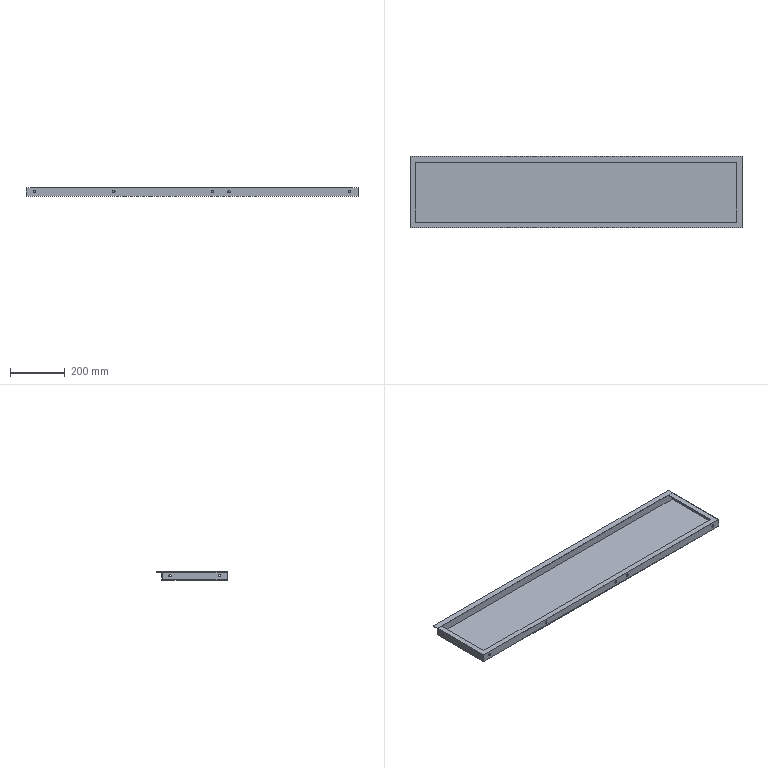Part | SolidWorks | features ICE 3, Extrusion 1, Shell 1 | 1 solid | 35 faces | box 1210 x 260 x 30 mm | volume 849119 mm3 | cylinder 18 | plane 17 | commonest cylinder face diameters 9 x18
STEP:
#1=CARTESIAN_POINT('',(740.,0.,11.5));
#2=VERTEX_POINT('',#1);
#3=CARTESIAN_POINT('',(740.,0.,20.5));
#4=VERTEX_POINT('',#3);
#5=CARTESIAN_POINT('',(740.,0.,16.));
#6=DIRECTION('',(0.,1.,0.));
#7=DIRECTION('',(0.,0.,1.));
#8=AXIS2_PLACEMENT_3D('',#5,#6,#7);
#9=CIRCLE('',#8,4.5);
#10=EDGE_CURVE('',#2,#4,#9,.T.);
#11=ORIENTED_EDGE('',*,*,#10,.F.);
#12=CARTESIAN_POINT('',(740.,2.,11.5));
#13=VERTEX_POINT('',#12);
#14=CARTESIAN_POINT('',(740.,-43.,11.5));
#15=DIRECTION('',(0.,1.,0.));
#16=VECTOR('',#15,1000.);
#17=LINE('',#14,#16);
#18=EDGE_CURVE('',#2,#13,#17,.T.);
#19=ORIENTED_EDGE('',*,*,#18,.T.);
#20=CARTESIAN_POINT('',(740.,2.,20.5));
#21=VERTEX_POINT('',#20);
#22=CARTESIAN_POINT('',(740.,2.,16.));
#23=DIRECTION('',(0.,1.,0.));
#24=DIRECTION('',(0.,0.,1.));
#25=AXIS2_PLACEMENT_3D('',#22,#23,#24);
#26=CIRCLE('',#25,4.5);
#27=EDGE_CURVE('',#13,#21,#26,.T.);
#28=ORIENTED_EDGE('',*,*,#27,.T.);
#29=CARTESIAN_POINT('',(740.,-43.,20.5));
#30=DIRECTION('',(0.,1.,0.));
#31=VECTOR('',#30,1000.);
#32=LINE('',#29,#31);
#33=EDGE_CURVE('',#4,#21,#32,.T.);
#34=ORIENTED_EDGE('',*,*,#33,.F.);
#35=EDGE_LOOP('',(#11,#19,#28,#34));
#36=FACE_OUTER_BOUND('',#35,.T.);
#37=CARTESIAN_POINT('',(740.,-43.,16.));
#38=DIRECTION('',(0.,1.,0.));
#39=DIRECTION('',(0.,0.,1.));
#40=AXIS2_PLACEMENT_3D('',#37,#38,#39);
#41=CYLINDRICAL_SURFACE('',#40,4.5);
#42=ADVANCED_FACE('',(#36),#41,.F.);
#43=CARTESIAN_POINT('',(320.,0.,11.5));
#44=VERTEX_POINT('',#43);
#45=CARTESIAN_POINT('',(320.,0.,20.5));
#46=VERTEX_POINT('',#45);
#47=CARTESIAN_POINT('',(320.,0.,16.));
#48=DIRECTION('',(0.,1.,0.));
#49=DIRECTION('',(0.,0.,1.));
#50=AXIS2_PLACEMENT_3D('',#47,#48,#49);
#51=CIRCLE('',#50,4.5);
#52=EDGE_CURVE('',#44,#46,#51,.T.);
#53=ORIENTED_EDGE('',*,*,#52,.F.);
#54=CARTESIAN_POINT('',(320.,2.,11.5));
#55=VERTEX_POINT('',#54);
#56=CARTESIAN_POINT('',(320.,-43.,11.5));
#57=DIRECTION('',(0.,1.,0.));
#58=VECTOR('',#57,1000.);
#59=LINE('',#56,#58);
#60=EDGE_CURVE('',#44,#55,#59,.T.);
#61=ORIENTED_EDGE('',*,*,#60,.T.);
#62=CARTESIAN_POINT('',(320.,2.,20.5));
#63=VERTEX_POINT('',#62);
#64=CARTESIAN_POINT('',(320.,2.,16.));
#65=DIRECTION('',(0.,1.,0.));
#66=DIRECTION('',(0.,0.,1.));
#67=AXIS2_PLACEMENT_3D('',#64,#65,#66);
#68=CIRCLE('',#67,4.5);
#69=EDGE_CURVE('',#55,#63,#68,.T.);
#70=ORIENTED_EDGE('',*,*,#69,.T.);
#71=CARTESIAN_POINT('',(320.,-43.,20.5));
#72=DIRECTION('',(0.,1.,0.));
#73=VECTOR('',#72,1000.);
#74=LINE('',#71,#73);
#75=EDGE_CURVE('',#46,#63,#74,.T.);
#76=ORIENTED_EDGE('',*,*,#75,.F.);
#77=EDGE_LOOP('',(#53,#61,#70,#76));
#78=FACE_OUTER_BOUND('',#77,.T.);
#79=CARTESIAN_POINT('',(320.,-43.,16.));
#80=DIRECTION('',(0.,1.,0.));
#81=DIRECTION('',(0.,0.,1.));
#82=AXIS2_PLACEMENT_3D('',#79,#80,#81);
#83=CYLINDRICAL_SURFACE('',#82,4.5);
#84=ADVANCED_FACE('',(#78),#83,.F.);
#85=CARTESIAN_POINT('',(680.,0.,11.5));
#86=VERTEX_POINT('',#85);
#87=CARTESIAN_POINT('',(680.,0.,20.5));
#88=VERTEX_POINT('',#87);
#89=CARTESIAN_POINT('',(680.,0.,16.));
#90=DIRECTION('',(0.,1.,0.));
#91=DIRECTION('',(0.,0.,1.));
#92=AXIS2_PLACEMENT_3D('',#89,#90,#91);
#93=CIRCLE('',#92,4.5);
#94=EDGE_CURVE('',#86,#88,#93,.T.);
#95=ORIENTED_EDGE('',*,*,#94,.F.);
#96=CARTESIAN_POINT('',(680.,2.,11.5));
#97=VERTEX_POINT('',#96);
#98=CARTESIAN_POINT('',(680.,-43.,11.5));
#99=DIRECTION('',(0.,1.,0.));
#100=VECTOR('',#99,1000.);
#101=LINE('',#98,#100);
#102=EDGE_CURVE('',#86,#97,#101,.T.);
#103=ORIENTED_EDGE('',*,*,#102,.T.);
#104=CARTESIAN_POINT('',(680.,2.,20.5));
#105=VERTEX_POINT('',#104);
#106=CARTESIAN_POINT('',(680.,2.,16.));
#107=DIRECTION('',(0.,1.,0.));
#108=DIRECTION('',(0.,0.,1.));
#109=AXIS2_PLACEMENT_3D('',#106,#107,#108);
#110=CIRCLE('',#109,4.5);
#111=EDGE_CURVE('',#97,#105,#110,.T.);
#112=ORIENTED_EDGE('',*,*,#111,.T.);
#113=CARTESIAN_POINT('',(680.,-43.,20.5));
#114=DIRECTION('',(0.,1.,0.));
#115=VECTOR('',#114,1000.);
#116=LINE('',#113,#115);
#117=EDGE_CURVE('',#88,#105,#116,.T.);
#118=ORIENTED_EDGE('',*,*,#117,.F.);
#119=EDGE_LOOP('',(#95,#103,#112,#118));
#120=FACE_OUTER_BOUND('',#119,.T.);
#121=CARTESIAN_POINT('',(680.,-43.,16.));
#122=DIRECTION('',(0.,1.,0.));
#123=DIRECTION('',(0.,0.,1.));
#124=AXIS2_PLACEMENT_3D('',#121,#122,#123);
#125=CYLINDRICAL_SURFACE('',#124,4.5);
#126=ADVANCED_FACE('',(#120),#125,.F.);
#127=CARTESIAN_POINT('',(1180.,0.,11.5));
#128=VERTEX_POINT('',#127);
#129=CARTESIAN_POINT('',(1180.,0.,20.5));
#130=VERTEX_POINT('',#129);
#131=CARTESIAN_POINT('',(1180.,0.,16.));
#132=DIRECTION('',(0.,1.,0.));
#133=DIRECTION('',(0.,0.,1.));
#134=AXIS2_PLACEMENT_3D('',#131,#132,#133);
#135=CIRCLE('',#134,4.5);
#136=EDGE_CURVE('',#128,#130,#135,.T.);
#137=ORIENTED_EDGE('',*,*,#136,.F.);
#138=CARTESIAN_POINT('',(1180.,2.,11.5));
#139=VERTEX_POINT('',#138);
#140=CARTESIAN_POINT('',(1180.,-43.,11.5));
#141=DIRECTION('',(0.,1.,0.));
#142=VECTOR('',#141,1000.);
#143=LINE('',#140,#142);
#144=EDGE_CURVE('',#128,#139,#143,.T.);
#145=ORIENTED_EDGE('',*,*,#144,.T.);
#146=CARTESIAN_POINT('',(1180.,2.,20.5));
#147=VERTEX_POINT('',#146);
#148=CARTESIAN_POINT('',(1180.,2.,16.));
#149=DIRECTION('',(0.,1.,0.));
#150=DIRECTION('',(0.,0.,1.));
#151=AXIS2_PLACEMENT_3D('',#148,#149,#150);
#152=CIRCLE('',#151,4.5);
#153=EDGE_CURVE('',#139,#147,#152,.T.);
#154=ORIENTED_EDGE('',*,*,#153,.T.);
#155=CARTESIAN_POINT('',(1180.,-43.,20.5));
#156=DIRECTION('',(0.,1.,0.));
#157=VECTOR('',#156,1000.);
#158=LINE('',#155,#157);
#159=EDGE_CURVE('',#130,#147,#158,.T.);
#160=ORIENTED_EDGE('',*,*,#159,.F.);
#161=EDGE_LOOP('',(#137,#145,#154,#160));
#162=FACE_OUTER_BOUND('',#161,.T.);
#163=CARTESIAN_POINT('',(1180.,-43.,16.));
#164=DIRECTION('',(0.,1.,0.));
#165=DIRECTION('',(0.,0.,1.));
#166=AXIS2_PLACEMENT_3D('',#163,#164,#165);
#167=CYLINDRICAL_SURFACE('',#166,4.5);
#168=ADVANCED_FACE('',(#162),#167,.F.);
#169=CARTESIAN_POINT('',(30.,0.,11.5));
#170=VERTEX_POINT('',#169);
#171=CARTESIAN_POINT('',(30.,0.,20.5));
#172=VERTEX_POINT('',#171);
#173=CARTESIAN_POINT('',(30.,0.,16.));
#174=DIRECTION('',(0.,1.,0.));
#175=DIRECTION('',(0.,0.,1.));
#176=AXIS2_PLACEMENT_3D('',#173,#174,#175);
#177=CIRCLE('',#176,4.5);
#178=EDGE_CURVE('',#170,#172,#177,.T.);
#179=ORIENTED_EDGE('',*,*,#178,.F.);
#180=CARTESIAN_POINT('',(30.,2.,11.5));
#181=VERTEX_POINT('',#180);
#182=CARTESIAN_POINT('',(30.,-43.,11.5));
#183=DIRECTION('',(0.,1.,0.));
#184=VECTOR('',#183,1000.);
#185=LINE('',#182,#184);
#186=EDGE_CURVE('',#170,#181,#185,.T.);
#187=ORIENTED_EDGE('',*,*,#186,.T.);
#188=CARTESIAN_POINT('',(30.,2.,20.5));
#189=VERTEX_POINT('',#188);
#190=CARTESIAN_POINT('',(30.,2.,16.));
#191=DIRECTION('',(0.,1.,0.));
#192=DIRECTION('',(0.,0.,1.));
#193=AXIS2_PLACEMENT_3D('',#190,#191,#192);
#194=CIRCLE('',#193,4.5);
#195=EDGE_CURVE('',#181,#189,#194,.T.);
#196=ORIENTED_EDGE('',*,*,#195,.T.);
#197=CARTESIAN_POINT('',(30.,-43.,20.5));
#198=DIRECTION('',(0.,1.,0.));
#199=VECTOR('',#198,1000.);
#200=LINE('',#197,#199);
#201=EDGE_CURVE('',#172,#189,#200,.T.);
#202=ORIENTED_EDGE('',*,*,#201,.F.);
#203=EDGE_LOOP('',(#179,#187,#196,#202));
#204=FACE_OUTER_BOUND('',#203,.T.);
#205=CARTESIAN_POINT('',(30.,-43.,16.));
#206=DIRECTION('',(0.,1.,0.));
#207=DIRECTION('',(0.,0.,1.));
#208=AXIS2_PLACEMENT_3D('',#205,#206,#207);
#209=CYLINDRICAL_SURFACE('',#208,4.5);
#210=ADVANCED_FACE('',(#204),#209,.F.);
#211=CARTESIAN_POINT('',(0.,210.,20.5));
#212=VERTEX_POINT('',#211);
#213=CARTESIAN_POINT('',(0.,210.,11.5));
#214=VERTEX_POINT('',#213);
#215=CARTESIAN_POINT('',(0.,210.,16.));
#216=DIRECTION('',(1.,0.,0.));
#217=DIRECTION('',(0.,0.,-1.));
#218=AXIS2_PLACEMENT_3D('',#215,#216,#217);
#219=CIRCLE('',#218,4.5);
#220=EDGE_CURVE('',#212,#214,#219,.T.);
#221=ORIENTED_EDGE('',*,*,#220,.F.);
#222=CARTESIAN_POINT('',(2.,210.,20.5));
#223=VERTEX_POINT('',#222);
#224=CARTESIAN_POINT('',(-196.,210.,20.5));
#225=DIRECTION('',(1.,0.,0.));
#226=VECTOR('',#225,1000.);
#227=LINE('',#224,#226);
#228=EDGE_CURVE('',#212,#223,#227,.T.);
#229=ORIENTED_EDGE('',*,*,#228,.T.);
#230=CARTESIAN_POINT('',(2.,210.,11.5));
#231=VERTEX_POINT('',#230);
#232=CARTESIAN_POINT('',(2.,210.,16.));
#233=DIRECTION('',(1.,0.,0.));
#234=DIRECTION('',(0.,0.,-1.));
#235=AXIS2_PLACEMENT_3D('',#232,#233,#234);
#236=CIRCLE('',#235,4.5);
#237=EDGE_CURVE('',#223,#231,#236,.T.);
#238=ORIENTED_EDGE('',*,*,#237,.T.);
#239=CARTESIAN_POINT('',(-196.,210.,11.5));
#240=DIRECTION('',(1.,0.,0.));
#241=VECTOR('',#240,1000.);
#242=LINE('',#239,#241);
#243=EDGE_CURVE('',#214,#231,#242,.T.);
#244=ORIENTED_EDGE('',*,*,#243,.F.);
#245=EDGE_LOOP('',(#221,#229,#238,#244));
#246=FACE_OUTER_BOUND('',#245,.T.);
#247=CARTESIAN_POINT('',(-196.,210.,16.));
#248=DIRECTION('',(1.,0.,0.));
#249=DIRECTION('',(0.,0.,-1.));
#250=AXIS2_PLACEMENT_3D('',#247,#248,#249);
#251=CYLINDRICAL_SURFACE('',#250,4.5);
#252=ADVANCED_FACE('',(#246),#251,.F.);
#253=CARTESIAN_POINT('',(1208.,210.,11.5));
#254=VERTEX_POINT('',#253);
#255=CARTESIAN_POINT('',(1208.,210.,20.5));
#256=VERTEX_POINT('',#255);
#257=CARTESIAN_POINT('',(1208.,210.,16.));
#258=DIRECTION('',(-1.,0.,0.));
#259=DIRECTION('',(0.,0.,1.));
#260=AXIS2_PLACEMENT_3D('',#257,#258,#259);
#261=CIRCLE('',#260,4.5);
#262=EDGE_CURVE('',#254,#256,#261,.T.);
#263=ORIENTED_EDGE('',*,*,#262,.T.);
#264=CARTESIAN_POINT('',(1210.,210.,20.5));
#265=VERTEX_POINT('',#264);
#266=CARTESIAN_POINT('',(-196.,210.,20.5));
#267=DIRECTION('',(1.,0.,0.));
#268=VECTOR('',#267,1000.);
#269=LINE('',#266,#268);
#270=EDGE_CURVE('',#256,#265,#269,.T.);
#271=ORIENTED_EDGE('',*,*,#270,.T.);
#272=CARTESIAN_POINT('',(1210.,210.,11.5));
#273=VERTEX_POINT('',#272);
#274=CARTESIAN_POINT('',(1210.,210.,16.));
#275=DIRECTION('',(-1.,0.,0.));
#276=DIRECTION('',(0.,0.,1.));
#277=AXIS2_PLACEMENT_3D('',#274,#275,#276);
#278=CIRCLE('',#277,4.5);
#279=EDGE_CURVE('',#273,#265,#278,.T.);
#280=ORIENTED_EDGE('',*,*,#279,.F.);
#281=CARTESIAN_POINT('',(-196.,210.,11.5));
#282=DIRECTION('',(1.,0.,0.));
#283=VECTOR('',#282,1000.);
#284=LINE('',#281,#283);
#285=EDGE_CURVE('',#254,#273,#284,.T.);
#286=ORIENTED_EDGE('',*,*,#285,.F.);
#287=EDGE_LOOP('',(#263,#271,#280,#286));
#288=FACE_OUTER_BOUND('',#287,.T.);
#289=CARTESIAN_POINT('',(-196.,210.,16.));
#290=DIRECTION('',(1.,0.,0.));
#291=DIRECTION('',(0.,0.,-1.));
#292=AXIS2_PLACEMENT_3D('',#289,#290,#291);
#293=CYLINDRICAL_SURFACE('',#292,4.5);
#294=ADVANCED_FACE('',(#288),#293,.F.);
#295=CARTESIAN_POINT('',(0.,30.,20.5));
#296=VERTEX_POINT('',#295);
#297=CARTESIAN_POINT('',(0.,30.,11.5));
#298=VERTEX_POINT('',#297);
#299=CARTESIAN_POINT('',(0.,30.,16.));
#300=DIRECTION('',(1.,0.,0.));
#301=DIRECTION('',(0.,0.,-1.));
#302=AXIS2_PLACEMENT_3D('',#299,#300,#301);
#303=CIRCLE('',#302,4.5);
#304=EDGE_CURVE('',#296,#298,#303,.T.);
#305=ORIENTED_EDGE('',*,*,#304,.F.);
#306=CARTESIAN_POINT('',(2.,30.,20.5));
#307=VERTEX_POINT('',#306);
#308=CARTESIAN_POINT('',(-196.,30.,20.5));
#309=DIRECTION('',(1.,0.,0.));
#310=VECTOR('',#309,1000.);
#311=LINE('',#308,#310);
#312=EDGE_CURVE('',#296,#307,#311,.T.);
#313=ORIENTED_EDGE('',*,*,#312,.T.);
#314=CARTESIAN_POINT('',(2.,30.,11.5));
#315=VERTEX_POINT('',#314);
#316=CARTESIAN_POINT('',(2.,30.,16.));
#317=DIRECTION('',(1.,0.,0.));
#318=DIRECTION('',(0.,0.,-1.));
#319=AXIS2_PLACEMENT_3D('',#316,#317,#318);
#320=CIRCLE('',#319,4.5);
#321=EDGE_CURVE('',#307,#315,#320,.T.);
#322=ORIENTED_EDGE('',*,*,#321,.T.);
#323=CARTESIAN_POINT('',(-196.,30.,11.5));
#324=DIRECTION('',(1.,0.,0.));
#325=VECTOR('',#324,1000.);
#326=LINE('',#323,#325);
#327=EDGE_CURVE('',#298,#315,#326,.T.);
#328=ORIENTED_EDGE('',*,*,#327,.F.);
#329=EDGE_LOOP('',(#305,#313,#322,#328));
#330=FACE_OUTER_BOUND('',#329,.T.);
#331=CARTESIAN_POINT('',(-196.,30.,16.));
#332=DIRECTION('',(1.,0.,0.));
#333=DIRECTION('',(0.,0.,-1.));
#334=AXIS2_PLACEMENT_3D('',#331,#332,#333);
#335=CYLINDRICAL_SURFACE('',#334,4.5);
#336=ADVANCED_FACE('',(#330),#335,.F.);
#337=CARTESIAN_POINT('',(1208.,30.,11.5));
#338=VERTEX_POINT('',#337);
#339=CARTESIAN_POINT('',(1208.,30.,20.5));
#340=VERTEX_POINT('',#339);
#341=CARTESIAN_POINT('',(1208.,30.,16.));
#342=DIRECTION('',(-1.,0.,0.));
#343=DIRECTION('',(0.,0.,1.));
#344=AXIS2_PLACEMENT_3D('',#341,#342,#343);
#345=CIRCLE('',#344,4.5);
#346=EDGE_CURVE('',#338,#340,#345,.T.);
#347=ORIENTED_EDGE('',*,*,#346,.T.);
#348=CARTESIAN_POINT('',(1210.,30.,20.5));
#349=VERTEX_POINT('',#348);
#350=CARTESIAN_POINT('',(-196.,30.,20.5));
#351=DIRECTION('',(1.,0.,0.));
#352=VECTOR('',#351,1000.);
#353=LINE('',#350,#352);
#354=EDGE_CURVE('',#340,#349,#353,.T.);
#355=ORIENTED_EDGE('',*,*,#354,.T.);
#356=CARTESIAN_POINT('',(1210.,30.,11.5));
#357=VERTEX_POINT('',#356);
#358=CARTESIAN_POINT('',(1210.,30.,16.));
#359=DIRECTION('',(-1.,0.,0.));
#360=DIRECTION('',(0.,0.,1.));
#361=AXIS2_PLACEMENT_3D('',#358,#359,#360);
#362=CIRCLE('',#361,4.5);
#363=EDGE_CURVE('',#357,#349,#362,.T.);
#364=ORIENTED_EDGE('',*,*,#363,.F.);
#365=CARTESIAN_POINT('',(-196.,30.,11.5));
#366=DIRECTION('',(1.,0.,0.));
#367=VECTOR('',#366,1000.);
#368=LINE('',#365,#367);
#369=EDGE_CURVE('',#338,#357,#368,.T.);
#370=ORIENTED_EDGE('',*,*,#369,.F.);
#371=EDGE_LOOP('',(#347,#355,#364,#370));
#372=FACE_OUTER_BOUND('',#371,.T.);
#373=CARTESIAN_POINT('',(-196.,30.,16.));
#374=DIRECTION('',(1.,0.,0.));
#375=DIRECTION('',(0.,0.,-1.));
#376=AXIS2_PLACEMENT_3D('',#373,#374,#375);
#377=CYLINDRICAL_SURFACE('',#376,4.5);
#378=ADVANCED_FACE('',(#372),#377,.F.);
#379=CARTESIAN_POINT('',(1210.,240.,28.));
#380=VERTEX_POINT('',#379);
#381=CARTESIAN_POINT('',(0.,240.,28.));
#382=VERTEX_POINT('',#381);
#383=CARTESIAN_POINT('',(0.,240.,28.));
#384=DIRECTION('',(-1.,0.,0.));
#385=VECTOR('',#384,1000.);
#386=LINE('',#383,#385);
#387=EDGE_CURVE('',#380,#382,#386,.T.);
#388=ORIENTED_EDGE('',*,*,#387,.F.);
#389=CARTESIAN_POINT('',(1210.,240.,0.));
#390=VERTEX_POINT('',#389);
#391=CARTESIAN_POINT('',(1210.,240.,30.));
#392=DIRECTION('',(0.,0.,-1.));
#393=VECTOR('',#392,1000.);
#394=LINE('',#391,#393);
#395=EDGE_CURVE('',#380,#390,#394,.T.);
#396=ORIENTED_EDGE('',*,*,#395,.T.);
#397=CARTESIAN_POINT('',(0.,240.,0.));
#398=VERTEX_POINT('',#397);
#399=CARTESIAN_POINT('',(0.,240.,0.));
#400=DIRECTION('',(-1.,0.,0.));
#401=VECTOR('',#400,1000.);
#402=LINE('',#399,#401);
#403=EDGE_CURVE('',#390,#398,#402,.T.);
#404=ORIENTED_EDGE('',*,*,#403,.T.);
#405=CARTESIAN_POINT('',(0.,240.,30.));
#406=DIRECTION('',(0.,0.,-1.));
#407=VECTOR('',#406,1000.);
#408=LINE('',#405,#407);
#409=EDGE_CURVE('',#382,#398,#408,.T.);
#410=ORIENTED_EDGE('',*,*,#409,.F.);
#411=EDGE_LOOP('',(#388,#396,#404,#410));
#412=FACE_OUTER_BOUND('',#411,.T.);
#413=CARTESIAN_POINT('',(0.,240.,30.));
#414=DIRECTION('',(0.,-1.,0.));
#415=DIRECTION('',(0.,0.,-1.));
#416=AXIS2_PLACEMENT_3D('',#413,#414,#415);
#417=PLANE('',#416);
#418=ADVANCED_FACE('',(#412),#417,.F.);
#419=CARTESIAN_POINT('',(2.,210.,16.));
#420=DIRECTION('',(1.,0.,0.));
#421=DIRECTION('',(0.,0.,-1.));
#422=AXIS2_PLACEMENT_3D('',#419,#420,#421);
#423=CIRCLE('',#422,4.5);
#424=EDGE_CURVE('',#231,#223,#423,.T.);
#425=ORIENTED_EDGE('',*,*,#424,.F.);
#426=ORIENTED_EDGE('',*,*,#237,.F.);
#427=EDGE_LOOP('',(#425,#426));
#428=FACE_BOUND('',#427,.T.);
#429=CARTESIAN_POINT('',(2.,30.,16.));
#430=DIRECTION('',(1.,0.,0.));
#431=DIRECTION('',(0.,0.,-1.));
#432=AXIS2_PLACEMENT_3D('',#429,#430,#431);
#433=CIRCLE('',#432,4.5);
#434=EDGE_CURVE('',#315,#307,#433,.T.);
#435=ORIENTED_EDGE('',*,*,#434,.F.);
#436=ORIENTED_EDGE('',*,*,#321,.F.);
#437=EDGE_LOOP('',(#435,#436));
#438=FACE_BOUND('',#437,.T.);
#439=CARTESIAN_POINT('',(2.,238.,28.));
#440=VERTEX_POINT('',#439);
#441=CARTESIAN_POINT('',(2.,238.,2.));
#442=VERTEX_POINT('',#441);
#443=CARTESIAN_POINT('',(2.,238.,30.));
#444=DIRECTION('',(0.,0.,-1.));
#445=VECTOR('',#444,1000.);
#446=LINE('',#443,#445);
#447=EDGE_CURVE('',#440,#442,#446,.T.);
#448=ORIENTED_EDGE('',*,*,#447,.F.);
#449=CARTESIAN_POINT('',(2.,2.,28.));
#450=VERTEX_POINT('',#449);
#451=CARTESIAN_POINT('',(2.,0.,28.));
#452=DIRECTION('',(0.,-1.,0.));
#453=VECTOR('',#452,1000.);
#454=LINE('',#451,#453);
#455=EDGE_CURVE('',#440,#450,#454,.T.);
#456=ORIENTED_EDGE('',*,*,#455,.T.);
#457=CARTESIAN_POINT('',(2.,2.,2.));
#458=VERTEX_POINT('',#457);
#459=CARTESIAN_POINT('',(2.,2.,30.));
#460=DIRECTION('',(0.,0.,-1.));
#461=VECTOR('',#460,1000.);
#462=LINE('',#459,#461);
#463=EDGE_CURVE('',#450,#458,#462,.T.);
#464=ORIENTED_EDGE('',*,*,#463,.T.);
#465=CARTESIAN_POINT('',(2.,240.,2.));
#466=DIRECTION('',(0.,-1.,0.));
#467=VECTOR('',#466,1000.);
#468=LINE('',#465,#467);
#469=EDGE_CURVE('',#442,#458,#468,.T.);
#470=ORIENTED_EDGE('',*,*,#469,.F.);
#471=EDGE_LOOP('',(#448,#456,#464,#470));
#472=FACE_OUTER_BOUND('',#471,.T.);
#473=CARTESIAN_POINT('',(2.,0.,30.));
#474=DIRECTION('',(1.,0.,0.));
#475=DIRECTION('',(0.,0.,-1.));
#476=AXIS2_PLACEMENT_3D('',#473,#474,#475);
#477=PLANE('',#476);
#478=ADVANCED_FACE('',(#428,#438,#472),#477,.T.);
#479=CARTESIAN_POINT('',(740.,2.,16.));
#480=DIRECTION('',(0.,1.,0.));
#481=DIRECTION('',(0.,0.,1.));
#482=AXIS2_PLACEMENT_3D('',#479,#480,#481);
#483=CIRCLE('',#482,4.5);
#484=EDGE_CURVE('',#21,#13,#483,.T.);
#485=ORIENTED_EDGE('',*,*,#484,.F.);
#486=ORIENTED_EDGE('',*,*,#27,.F.);
#487=EDGE_LOOP('',(#485,#486));
#488=FACE_BOUND('',#487,.T.);
#489=CARTESIAN_POINT('',(320.,2.,16.));
#490=DIRECTION('',(0.,1.,0.));
#491=DIRECTION('',(0.,0.,1.));
#492=AXIS2_PLACEMENT_3D('',#489,#490,#491);
#493=CIRCLE('',#492,4.5);
#494=EDGE_CURVE('',#63,#55,#493,.T.);
#495=ORIENTED_EDGE('',*,*,#494,.F.);
#496=ORIENTED_EDGE('',*,*,#69,.F.);
#497=EDGE_LOOP('',(#495,#496));
#498=FACE_BOUND('',#497,.T.);
#499=CARTESIAN_POINT('',(680.,2.,16.));
#500=DIRECTION('',(0.,1.,0.));
#501=DIRECTION('',(0.,0.,1.));
#502=AXIS2_PLACEMENT_3D('',#499,#500,#501);
#503=CIRCLE('',#502,4.5);
#504=EDGE_CURVE('',#105,#97,#503,.T.);
#505=ORIENTED_EDGE('',*,*,#504,.F.);
#506=ORIENTED_EDGE('',*,*,#111,.F.);
#507=EDGE_LOOP('',(#505,#506));
#508=FACE_BOUND('',#507,.T.);
#509=CARTESIAN_POINT('',(1180.,2.,16.));
#510=DIRECTION('',(0.,1.,0.));
#511=DIRECTION('',(0.,0.,1.));
#512=AXIS2_PLACEMENT_3D('',#509,#510,#511);
#513=CIRCLE('',#512,4.5);
#514=EDGE_CURVE('',#147,#139,#513,.T.);
#515=ORIENTED_EDGE('',*,*,#514,.F.);
#516=ORIENTED_EDGE('',*,*,#153,.F.);
#517=EDGE_LOOP('',(#515,#516));
#518=FACE_BOUND('',#517,.T.);
#519=CARTESIAN_POINT('',(30.,2.,16.));
#520=DIRECTION('',(0.,1.,0.));
#521=DIRECTION('',(0.,0.,1.));
#522=AXIS2_PLACEMENT_3D('',#519,#520,#521);
#523=CIRCLE('',#522,4.5);
#524=EDGE_CURVE('',#189,#181,#523,.T.);
#525=ORIENTED_EDGE('',*,*,#524,.F.);
#526=ORIENTED_EDGE('',*,*,#195,.F.);
#527=EDGE_LOOP('',(#525,#526));
#528=FACE_BOUND('',#527,.T.);
#529=ORIENTED_EDGE('',*,*,#463,.F.);
#530=CARTESIAN_POINT('',(1208.,2.,28.));
#531=VERTEX_POINT('',#530);
#532=CARTESIAN_POINT('',(0.,2.,28.));
#533=DIRECTION('',(1.,0.,0.));
#534=VECTOR('',#533,1000.);
#535=LINE('',#532,#534);
#536=EDGE_CURVE('',#450,#531,#535,.T.);
#537=ORIENTED_EDGE('',*,*,#536,.T.);
#538=CARTESIAN_POINT('',(1208.,2.,2.));
#539=VERTEX_POINT('',#538);
#540=CARTESIAN_POINT('',(1208.,2.,30.));
#541=DIRECTION('',(0.,0.,-1.));
#542=VECTOR('',#541,1000.);
#543=LINE('',#540,#542);
#544=EDGE_CURVE('',#531,#539,#543,.T.);
#545=ORIENTED_EDGE('',*,*,#544,.T.);
#546=CARTESIAN_POINT('',(0.,2.,2.));
#547=DIRECTION('',(1.,0.,0.));
#548=VECTOR('',#547,1000.);
#549=LINE('',#546,#548);
#550=EDGE_CURVE('',#458,#539,#549,.T.);
#551=ORIENTED_EDGE('',*,*,#550,.F.);
#552=EDGE_LOOP('',(#529,#537,#545,#551));
#553=FACE_OUTER_BOUND('',#552,.T.);
#554=CARTESIAN_POINT('',(0.,2.,30.));
#555=DIRECTION('',(0.,1.,0.));
#556=DIRECTION('',(0.,0.,1.));
#557=AXIS2_PLACEMENT_3D('',#554,#555,#556);
#558=PLANE('',#557);
#559=ADVANCED_FACE('',(#488,#498,#508,#518,#528,#553),#558,.T.);
#560=ORIENTED_EDGE('',*,*,#262,.F.);
#561=CARTESIAN_POINT('',(1208.,210.,16.));
#562=DIRECTION('',(-1.,0.,0.));
#563=DIRECTION('',(0.,0.,1.));
#564=AXIS2_PLACEMENT_3D('',#561,#562,#563);
#565=CIRCLE('',#564,4.5);
#566=EDGE_CURVE('',#256,#254,#565,.T.);
#567=ORIENTED_EDGE('',*,*,#566,.F.);
#568=EDGE_LOOP('',(#560,#567));
#569=FACE_BOUND('',#568,.T.);
#570=ORIENTED_EDGE('',*,*,#346,.F.);
#571=CARTESIAN_POINT('',(1208.,30.,16.));
#572=DIRECTION('',(-1.,0.,0.));
#573=DIRECTION('',(0.,0.,1.));
#574=AXIS2_PLACEMENT_3D('',#571,#572,#573);
#575=CIRCLE('',#574,4.5);
#576=EDGE_CURVE('',#340,#338,#575,.T.);
#577=ORIENTED_EDGE('',*,*,#576,.F.);
#578=EDGE_LOOP('',(#570,#577));
#579=FACE_BOUND('',#578,.T.);
#580=ORIENTED_EDGE('',*,*,#544,.F.);
#581=CARTESIAN_POINT('',(1208.,238.,28.));
#582=VERTEX_POINT('',#581);
#583=CARTESIAN_POINT('',(1208.,0.,28.));
#584=DIRECTION('',(0.,1.,0.));
#585=VECTOR('',#584,1000.);
#586=LINE('',#583,#585);
#587=EDGE_CURVE('',#531,#582,#586,.T.);
#588=ORIENTED_EDGE('',*,*,#587,.T.);
#589=CARTESIAN_POINT('',(1208.,238.,2.));
#590=VERTEX_POINT('',#589);
#591=CARTESIAN_POINT('',(1208.,238.,30.));
#592=DIRECTION('',(0.,0.,-1.));
#593=VECTOR('',#592,1000.);
#594=LINE('',#591,#593);
#595=EDGE_CURVE('',#582,#590,#594,.T.);
#596=ORIENTED_EDGE('',*,*,#595,.T.);
#597=CARTESIAN_POINT('',(1208.,240.,2.));
#598=DIRECTION('',(0.,1.,0.));
#599=VECTOR('',#598,1000.);
#600=LINE('',#597,#599);
#601=EDGE_CURVE('',#539,#590,#600,.T.);
#602=ORIENTED_EDGE('',*,*,#601,.F.);
#603=EDGE_LOOP('',(#580,#588,#596,#602));
#604=FACE_OUTER_BOUND('',#603,.T.);
#605=CARTESIAN_POINT('',(1208.,0.,30.));
#606=DIRECTION('',(-1.,0.,0.));
#607=DIRECTION('',(0.,0.,1.));
#608=AXIS2_PLACEMENT_3D('',#605,#606,#607);
#609=PLANE('',#608);
#610=ADVANCED_FACE('',(#569,#579,#604),#609,.T.);
#611=CARTESIAN_POINT('',(1190.,238.,30.));
#612=VERTEX_POINT('',#611);
#613=CARTESIAN_POINT('',(20.,238.,30.));
#614=VERTEX_POINT('',#613);
#615=CARTESIAN_POINT('',(0.,238.,30.));
#616=DIRECTION('',(-1.,0.,0.));
#617=VECTOR('',#616,1000.);
#618=LINE('',#615,#617);
#619=EDGE_CURVE('',#612,#614,#618,.T.);
#620=ORIENTED_EDGE('',*,*,#619,.T.);
#621=CARTESIAN_POINT('',(20.,238.,28.));
#622=VERTEX_POINT('',#621);
#623=CARTESIAN_POINT('',(20.,238.,28.));
#624=DIRECTION('',(0.,0.,1.));
#625=VECTOR('',#624,1000.);
#626=LINE('',#623,#625);
#627=EDGE_CURVE('',#622,#614,#626,.T.);
#628=ORIENTED_EDGE('',*,*,#627,.F.);
#629=CARTESIAN_POINT('',(0.,238.,28.));
#630=DIRECTION('',(-1.,0.,0.));
#631=VECTOR('',#630,1000.);
#632=LINE('',#629,#631);
#633=EDGE_CURVE('',#622,#440,#632,.T.);
#634=ORIENTED_EDGE('',*,*,#633,.T.);
#635=ORIENTED_EDGE('',*,*,#447,.T.);
#636=CARTESIAN_POINT('',(0.,238.,2.));
#637=DIRECTION('',(-1.,0.,0.));
#638=VECTOR('',#637,1000.);
#639=LINE('',#636,#638);
#640=EDGE_CURVE('',#590,#442,#639,.T.);
#641=ORIENTED_EDGE('',*,*,#640,.F.);
#642=ORIENTED_EDGE('',*,*,#595,.F.);
#643=CARTESIAN_POINT('',(1190.,238.,28.));
#644=VERTEX_POINT('',#643);
#645=CARTESIAN_POINT('',(0.,238.,28.));
#646=DIRECTION('',(-1.,0.,0.));
#647=VECTOR('',#646,1000.);
#648=LINE('',#645,#647);
#649=EDGE_CURVE('',#582,#644,#648,.T.);
#650=ORIENTED_EDGE('',*,*,#649,.T.);
#651=CARTESIAN_POINT('',(1190.,238.,28.));
#652=DIRECTION('',(0.,0.,1.));
#653=VECTOR('',#652,1000.);
#654=LINE('',#651,#653);
#655=EDGE_CURVE('',#644,#612,#654,.T.);
#656=ORIENTED_EDGE('',*,*,#655,.T.);
#657=EDGE_LOOP('',(#620,#628,#634,#635,#641,#642,#650,#656));
#658=FACE_OUTER_BOUND('',#657,.T.);
#659=CARTESIAN_POINT('',(0.,238.,30.));
#660=DIRECTION('',(0.,-1.,0.));
#661=DIRECTION('',(0.,0.,-1.));
#662=AXIS2_PLACEMENT_3D('',#659,#660,#661);
#663=PLANE('',#662);
#664=ADVANCED_FACE('',(#658),#663,.T.);
#665=ORIENTED_EDGE('',*,*,#619,.F.);
#666=CARTESIAN_POINT('',(1190.,20.,30.));
#667=VERTEX_POINT('',#666);
#668=CARTESIAN_POINT('',(1190.,20.,30.));
#669=DIRECTION('',(0.,1.,0.));
#670=VECTOR('',#669,1000.);
#671=LINE('',#668,#670);
#672=EDGE_CURVE('',#667,#612,#671,.T.);
#673=ORIENTED_EDGE('',*,*,#672,.F.);
#674=CARTESIAN_POINT('',(20.,20.,30.));
#675=VERTEX_POINT('',#674);
#676=CARTESIAN_POINT('',(20.,20.,30.));
#677=DIRECTION('',(1.,0.,0.));
#678=VECTOR('',#677,1000.);
#679=LINE('',#676,#678);
#680=EDGE_CURVE('',#675,#667,#679,.T.);
#681=ORIENTED_EDGE('',*,*,#680,.F.);
#682=CARTESIAN_POINT('',(20.,20.,30.));
#683=DIRECTION('',(0.,-1.,0.));
#684=VECTOR('',#683,1000.);
#685=LINE('',#682,#684);
#686=EDGE_CURVE('',#614,#675,#685,.T.);
#687=ORIENTED_EDGE('',*,*,#686,.F.);
#688=EDGE_LOOP('',(#665,#673,#681,#687));
#689=FACE_BOUND('',#688,.T.);
#690=CARTESIAN_POINT('',(0.,260.,30.));
#691=VERTEX_POINT('',#690);
#692=CARTESIAN_POINT('',(0.,0.,30.));
#693=VERTEX_POINT('',#692);
#694=CARTESIAN_POINT('',(0.,0.,30.));
#695=DIRECTION('',(0.,-1.,0.));
#696=VECTOR('',#695,1000.);
#697=LINE('',#694,#696);
#698=EDGE_CURVE('',#691,#693,#697,.T.);
#699=ORIENTED_EDGE('',*,*,#698,.T.);
#700=CARTESIAN_POINT('',(1210.,0.,30.));
#701=VERTEX_POINT('',#700);
#702=CARTESIAN_POINT('',(0.,0.,30.));
#703=DIRECTION('',(1.,0.,0.));
#704=VECTOR('',#703,1000.);
#705=LINE('',#702,#704);
#706=EDGE_CURVE('',#693,#701,#705,.T.);
#707=ORIENTED_EDGE('',*,*,#706,.T.);
#708=CARTESIAN_POINT('',(1210.,260.,30.));
#709=VERTEX_POINT('',#708);
#710=CARTESIAN_POINT('',(1210.,0.,30.));
#711=DIRECTION('',(0.,1.,0.));
#712=VECTOR('',#711,1000.);
#713=LINE('',#710,#712);
#714=EDGE_CURVE('',#701,#709,#713,.T.);
#715=ORIENTED_EDGE('',*,*,#714,.T.);
#716=CARTESIAN_POINT('',(0.,260.,30.));
#717=DIRECTION('',(-1.,0.,0.));
#718=VECTOR('',#717,1000.);
#719=LINE('',#716,#718);
#720=EDGE_CURVE('',#709,#691,#719,.T.);
#721=ORIENTED_EDGE('',*,*,#720,.T.);
#722=EDGE_LOOP('',(#699,#707,#715,#721));
#723=FACE_OUTER_BOUND('',#722,.T.);
#724=CARTESIAN_POINT('',(0.,240.,30.));
#725=DIRECTION('',(0.,0.,-1.));
#726=DIRECTION('',(-1.,0.,0.));
#727=AXIS2_PLACEMENT_3D('',#724,#725,#726);
#728=PLANE('',#727);
#729=ADVANCED_FACE('',(#689,#723),#728,.F.);
#730=CARTESIAN_POINT('',(0.,210.,16.));
#731=DIRECTION('',(1.,0.,0.));
#732=DIRECTION('',(0.,0.,-1.));
#733=AXIS2_PLACEMENT_3D('',#730,#731,#732);
#734=CIRCLE('',#733,4.5);
#735=EDGE_CURVE('',#214,#212,#734,.T.);
#736=ORIENTED_EDGE('',*,*,#735,.T.);
#737=ORIENTED_EDGE('',*,*,#220,.T.);
#738=EDGE_LOOP('',(#736,#737));
#739=FACE_BOUND('',#738,.T.);
#740=CARTESIAN_POINT('',(0.,30.,16.));
#741=DIRECTION('',(1.,0.,0.));
#742=DIRECTION('',(0.,0.,-1.));
#743=AXIS2_PLACEMENT_3D('',#740,#741,#742);
#744=CIRCLE('',#743,4.5);
#745=EDGE_CURVE('',#298,#296,#744,.T.);
#746=ORIENTED_EDGE('',*,*,#745,.T.);
#747=ORIENTED_EDGE('',*,*,#304,.T.);
#748=EDGE_LOOP('',(#746,#747));
#749=FACE_BOUND('',#748,.T.);
#750=ORIENTED_EDGE('',*,*,#698,.F.);
#751=CARTESIAN_POINT('',(0.,260.,28.));
#752=VERTEX_POINT('',#751);
#753=CARTESIAN_POINT('',(0.,260.,28.));
#754=DIRECTION('',(0.,0.,1.));
#755=VECTOR('',#754,1000.);
#756=LINE('',#753,#755);
#757=EDGE_CURVE('',#752,#691,#756,.T.);
#758=ORIENTED_EDGE('',*,*,#757,.F.);
#759=CARTESIAN_POINT('',(0.,260.,28.));
#760=DIRECTION('',(0.,-1.,0.));
#761=VECTOR('',#760,1000.);
#762=LINE('',#759,#761);
#763=EDGE_CURVE('',#752,#382,#762,.T.);
#764=ORIENTED_EDGE('',*,*,#763,.T.);
#765=ORIENTED_EDGE('',*,*,#409,.T.);
#766=CARTESIAN_POINT('',(0.,0.,0.));
#767=VERTEX_POINT('',#766);
#768=CARTESIAN_POINT('',(0.,0.,0.));
#769=DIRECTION('',(0.,-1.,0.));
#770=VECTOR('',#769,1000.);
#771=LINE('',#768,#770);
#772=EDGE_CURVE('',#398,#767,#771,.T.);
#773=ORIENTED_EDGE('',*,*,#772,.T.);
#774=CARTESIAN_POINT('',(0.,0.,30.));
#775=DIRECTION('',(0.,0.,-1.));
#776=VECTOR('',#775,1000.);
#777=LINE('',#774,#776);
#778=EDGE_CURVE('',#693,#767,#777,.T.);
#779=ORIENTED_EDGE('',*,*,#778,.F.);
#780=EDGE_LOOP('',(#750,#758,#764,#765,#773,#779));
#781=FACE_OUTER_BOUND('',#780,.T.);
#782=CARTESIAN_POINT('',(0.,0.,30.));
#783=DIRECTION('',(1.,0.,0.));
#784=DIRECTION('',(0.,0.,-1.));
#785=AXIS2_PLACEMENT_3D('',#782,#783,#784);
#786=PLANE('',#785);
#787=ADVANCED_FACE('',(#739,#749,#781),#786,.F.);
#788=CARTESIAN_POINT('',(740.,0.,16.));
#789=DIRECTION('',(0.,1.,0.));
#790=DIRECTION('',(0.,0.,1.));
#791=AXIS2_PLACEMENT_3D('',#788,#789,#790);
#792=CIRCLE('',#791,4.5);
#793=EDGE_CURVE('',#4,#2,#792,.T.);
#794=ORIENTED_EDGE('',*,*,#793,.T.);
#795=ORIENTED_EDGE('',*,*,#10,.T.);
#796=EDGE_LOOP('',(#794,#795));
#797=FACE_BOUND('',#796,.T.);
#798=CARTESIAN_POINT('',(320.,0.,16.));
#799=DIRECTION('',(0.,1.,0.));
#800=DIRECTION('',(0.,0.,1.));
#801=AXIS2_PLACEMENT_3D('',#798,#799,#800);
#802=CIRCLE('',#801,4.5);
#803=EDGE_CURVE('',#46,#44,#802,.T.);
#804=ORIENTED_EDGE('',*,*,#803,.T.);
#805=ORIENTED_EDGE('',*,*,#52,.T.);
#806=EDGE_LOOP('',(#804,#805));
#807=FACE_BOUND('',#806,.T.);
#808=CARTESIAN_POINT('',(680.,0.,16.));
#809=DIRECTION('',(0.,1.,0.));
#810=DIRECTION('',(0.,0.,1.));
#811=AXIS2_PLACEMENT_3D('',#808,#809,#810);
#812=CIRCLE('',#811,4.5);
#813=EDGE_CURVE('',#88,#86,#812,.T.);
#814=ORIENTED_EDGE('',*,*,#813,.T.);
#815=ORIENTED_EDGE('',*,*,#94,.T.);
#816=EDGE_LOOP('',(#814,#815));
#817=FACE_BOUND('',#816,.T.);
#818=CARTESIAN_POINT('',(1180.,0.,16.));
#819=DIRECTION('',(0.,1.,0.));
#820=DIRECTION('',(0.,0.,1.));
#821=AXIS2_PLACEMENT_3D('',#818,#819,#820);
#822=CIRCLE('',#821,4.5);
#823=EDGE_CURVE('',#130,#128,#822,.T.);
#824=ORIENTED_EDGE('',*,*,#823,.T.);
#825=ORIENTED_EDGE('',*,*,#136,.T.);
#826=EDGE_LOOP('',(#824,#825));
#827=FACE_BOUND('',#826,.T.);
#828=CARTESIAN_POINT('',(30.,0.,16.));
#829=DIRECTION('',(0.,1.,0.));
#830=DIRECTION('',(0.,0.,1.));
#831=AXIS2_PLACEMENT_3D('',#828,#829,#830);
#832=CIRCLE('',#831,4.5);
#833=EDGE_CURVE('',#172,#170,#832,.T.);
#834=ORIENTED_EDGE('',*,*,#833,.T.);
#835=ORIENTED_EDGE('',*,*,#178,.T.);
#836=EDGE_LOOP('',(#834,#835));
#837=FACE_BOUND('',#836,.T.);
#838=ORIENTED_EDGE('',*,*,#778,.T.);
#839=CARTESIAN_POINT('',(1210.,0.,0.));
#840=VERTEX_POINT('',#839);
#841=CARTESIAN_POINT('',(0.,0.,0.));
#842=DIRECTION('',(1.,0.,0.));
#843=VECTOR('',#842,1000.);
#844=LINE('',#841,#843);
#845=EDGE_CURVE('',#767,#840,#844,.T.);
#846=ORIENTED_EDGE('',*,*,#845,.T.);
#847=CARTESIAN_POINT('',(1210.,0.,30.));
#848=DIRECTION('',(0.,0.,-1.));
#849=VECTOR('',#848,1000.);
#850=LINE('',#847,#849);
#851=EDGE_CURVE('',#701,#840,#850,.T.);
#852=ORIENTED_EDGE('',*,*,#851,.F.);
#853=ORIENTED_EDGE('',*,*,#706,.F.);
#854=EDGE_LOOP('',(#838,#846,#852,#853));
#855=FACE_OUTER_BOUND('',#854,.T.);
#856=CARTESIAN_POINT('',(0.,0.,30.));
#857=DIRECTION('',(0.,1.,0.));
#858=DIRECTION('',(0.,0.,1.));
#859=AXIS2_PLACEMENT_3D('',#856,#857,#858);
#860=PLANE('',#859);
#861=ADVANCED_FACE('',(#797,#807,#817,#827,#837,#855),#860,.F.);
#862=ORIENTED_EDGE('',*,*,#279,.T.);
#863=CARTESIAN_POINT('',(1210.,210.,16.));
#864=DIRECTION('',(-1.,0.,0.));
#865=DIRECTION('',(0.,0.,1.));
#866=AXIS2_PLACEMENT_3D('',#863,#864,#865);
#867=CIRCLE('',#866,4.5);
#868=EDGE_CURVE('',#265,#273,#867,.T.);
#869=ORIENTED_EDGE('',*,*,#868,.T.);
#870=EDGE_LOOP('',(#862,#869));
#871=FACE_BOUND('',#870,.T.);
#872=ORIENTED_EDGE('',*,*,#363,.T.);
#873=CARTESIAN_POINT('',(1210.,30.,16.));
#874=DIRECTION('',(-1.,0.,0.));
#875=DIRECTION('',(0.,0.,1.));
#876=AXIS2_PLACEMENT_3D('',#873,#874,#875);
#877=CIRCLE('',#876,4.5);
#878=EDGE_CURVE('',#349,#357,#877,.T.);
#879=ORIENTED_EDGE('',*,*,#878,.T.);
#880=EDGE_LOOP('',(#872,#879));
#881=FACE_BOUND('',#880,.T.);
#882=ORIENTED_EDGE('',*,*,#851,.T.);
#883=CARTESIAN_POINT('',(1210.,0.,0.));
#884=DIRECTION('',(0.,1.,0.));
#885=VECTOR('',#884,1000.);
#886=LINE('',#883,#885);
#887=EDGE_CURVE('',#840,#390,#886,.T.);
#888=ORIENTED_EDGE('',*,*,#887,.T.);
#889=ORIENTED_EDGE('',*,*,#395,.F.);
#890=CARTESIAN_POINT('',(1210.,260.,28.));
#891=VERTEX_POINT('',#890);
#892=CARTESIAN_POINT('',(1210.,260.,28.));
#893=DIRECTION('',(0.,1.,0.));
#894=VECTOR('',#893,1000.);
#895=LINE('',#892,#894);
#896=EDGE_CURVE('',#380,#891,#895,.T.);
#897=ORIENTED_EDGE('',*,*,#896,.T.);
#898=CARTESIAN_POINT('',(1210.,260.,28.));
#899=DIRECTION('',(0.,0.,1.));
#900=VECTOR('',#899,1000.);
#901=LINE('',#898,#900);
#902=EDGE_CURVE('',#891,#709,#901,.T.);
#903=ORIENTED_EDGE('',*,*,#902,.T.);
#904=ORIENTED_EDGE('',*,*,#714,.F.);
#905=EDGE_LOOP('',(#882,#888,#889,#897,#903,#904));
#906=FACE_OUTER_BOUND('',#905,.T.);
#907=CARTESIAN_POINT('',(1210.,0.,30.));
#908=DIRECTION('',(-1.,0.,0.));
#909=DIRECTION('',(0.,0.,1.));
#910=AXIS2_PLACEMENT_3D('',#907,#908,#909);
#911=PLANE('',#910);
#912=ADVANCED_FACE('',(#871,#881,#906),#911,.F.);
#913=ORIENTED_EDGE('',*,*,#772,.F.);
#914=ORIENTED_EDGE('',*,*,#403,.F.);
#915=ORIENTED_EDGE('',*,*,#887,.F.);
#916=ORIENTED_EDGE('',*,*,#845,.F.);
#917=EDGE_LOOP('',(#913,#914,#915,#916));
#918=FACE_OUTER_BOUND('',#917,.T.);
#919=CARTESIAN_POINT('',(0.,240.,0.));
#920=DIRECTION('',(0.,0.,-1.));
#921=DIRECTION('',(-1.,0.,0.));
#922=AXIS2_PLACEMENT_3D('',#919,#920,#921);
#923=PLANE('',#922);
#924=ADVANCED_FACE('',(#918),#923,.T.);
#925=ORIENTED_EDGE('',*,*,#469,.T.);
#926=ORIENTED_EDGE('',*,*,#550,.T.);
#927=ORIENTED_EDGE('',*,*,#601,.T.);
#928=ORIENTED_EDGE('',*,*,#640,.T.);
#929=EDGE_LOOP('',(#925,#926,#927,#928));
#930=FACE_OUTER_BOUND('',#929,.T.);
#931=CARTESIAN_POINT('',(0.,240.,2.));
#932=DIRECTION('',(0.,0.,-1.));
#933=DIRECTION('',(-1.,0.,0.));
#934=AXIS2_PLACEMENT_3D('',#931,#932,#933);
#935=PLANE('',#934);
#936=ADVANCED_FACE('',(#930),#935,.F.);
#937=ORIENTED_EDGE('',*,*,#680,.T.);
#938=CARTESIAN_POINT('',(1190.,20.,28.));
#939=VERTEX_POINT('',#938);
#940=CARTESIAN_POINT('',(1190.,20.,28.));
#941=DIRECTION('',(0.,0.,1.));
#942=VECTOR('',#941,1000.);
#943=LINE('',#940,#942);
#944=EDGE_CURVE('',#939,#667,#943,.T.);
#945=ORIENTED_EDGE('',*,*,#944,.F.);
#946=CARTESIAN_POINT('',(20.,20.,28.));
#947=VERTEX_POINT('',#946);
#948=CARTESIAN_POINT('',(20.,20.,28.));
#949=DIRECTION('',(1.,0.,0.));
#950=VECTOR('',#949,1000.);
#951=LINE('',#948,#950);
#952=EDGE_CURVE('',#947,#939,#951,.T.);
#953=ORIENTED_EDGE('',*,*,#952,.F.);
#954=CARTESIAN_POINT('',(20.,20.,28.));
#955=DIRECTION('',(0.,0.,1.));
#956=VECTOR('',#955,1000.);
#957=LINE('',#954,#956);
#958=EDGE_CURVE('',#947,#675,#957,.T.);
#959=ORIENTED_EDGE('',*,*,#958,.T.);
#960=EDGE_LOOP('',(#937,#945,#953,#959));
#961=FACE_OUTER_BOUND('',#960,.T.);
#962=CARTESIAN_POINT('',(20.,20.,28.));
#963=DIRECTION('',(0.,-1.,0.));
#964=DIRECTION('',(1.,0.,0.));
#965=AXIS2_PLACEMENT_3D('',#962,#963,#964);
#966=PLANE('',#965);
#967=ADVANCED_FACE('',(#961),#966,.F.);
#968=ORIENTED_EDGE('',*,*,#686,.T.);
#969=ORIENTED_EDGE('',*,*,#958,.F.);
#970=CARTESIAN_POINT('',(20.,20.,28.));
#971=DIRECTION('',(0.,-1.,0.));
#972=VECTOR('',#971,1000.);
#973=LINE('',#970,#972);
#974=EDGE_CURVE('',#622,#947,#973,.T.);
#975=ORIENTED_EDGE('',*,*,#974,.F.);
#976=ORIENTED_EDGE('',*,*,#627,.T.);
#977=EDGE_LOOP('',(#968,#969,#975,#976));
#978=FACE_OUTER_BOUND('',#977,.T.);
#979=CARTESIAN_POINT('',(20.,20.,28.));
#980=DIRECTION('',(-1.,0.,0.));
#981=DIRECTION('',(0.,-1.,0.));
#982=AXIS2_PLACEMENT_3D('',#979,#980,#981);
#983=PLANE('',#982);
#984=ADVANCED_FACE('',(#978),#983,.F.);
#985=ORIENTED_EDGE('',*,*,#672,.T.);
#986=ORIENTED_EDGE('',*,*,#655,.F.);
#987=CARTESIAN_POINT('',(1190.,20.,28.));
#988=DIRECTION('',(0.,1.,0.));
#989=VECTOR('',#988,1000.);
#990=LINE('',#987,#989);
#991=EDGE_CURVE('',#939,#644,#990,.T.);
#992=ORIENTED_EDGE('',*,*,#991,.F.);
#993=ORIENTED_EDGE('',*,*,#944,.T.);
#994=EDGE_LOOP('',(#985,#986,#992,#993));
#995=FACE_OUTER_BOUND('',#994,.T.);
#996=CARTESIAN_POINT('',(1190.,20.,28.));
#997=DIRECTION('',(1.,0.,0.));
#998=DIRECTION('',(0.,0.,-1.));
#999=AXIS2_PLACEMENT_3D('',#996,#997,#998);
#1000=PLANE('',#999);
#1001=ADVANCED_FACE('',(#995),#1000,.F.);
#1002=ORIENTED_EDGE('',*,*,#649,.F.);
#1003=ORIENTED_EDGE('',*,*,#587,.F.);
#1004=ORIENTED_EDGE('',*,*,#536,.F.);
#1005=ORIENTED_EDGE('',*,*,#455,.F.);
#1006=ORIENTED_EDGE('',*,*,#633,.F.);
#1007=ORIENTED_EDGE('',*,*,#974,.T.);
#1008=ORIENTED_EDGE('',*,*,#952,.T.);
#1009=ORIENTED_EDGE('',*,*,#991,.T.);
#1010=EDGE_LOOP('',(#1002,#1003,#1004,#1005,#1006,#1007,#1008,#1009));
#1011=FACE_OUTER_BOUND('',#1010,.T.);
#1012=CARTESIAN_POINT('',(0.,0.,28.));
#1013=DIRECTION('',(0.,0.,1.));
#1014=DIRECTION('',(1.,0.,0.));
#1015=AXIS2_PLACEMENT_3D('',#1012,#1013,#1014);
#1016=PLANE('',#1015);
#1017=ADVANCED_FACE('',(#1011),#1016,.F.);
#1018=ORIENTED_EDGE('',*,*,#896,.F.);
#1019=ORIENTED_EDGE('',*,*,#387,.T.);
#1020=ORIENTED_EDGE('',*,*,#763,.F.);
#1021=CARTESIAN_POINT('',(0.,260.,28.));
#1022=DIRECTION('',(-1.,0.,0.));
#1023=VECTOR('',#1022,1000.);
#1024=LINE('',#1021,#1023);
#1025=EDGE_CURVE('',#891,#752,#1024,.T.);
#1026=ORIENTED_EDGE('',*,*,#1025,.F.);
#1027=EDGE_LOOP('',(#1018,#1019,#1020,#1026));
#1028=FACE_OUTER_BOUND('',#1027,.T.);
#1029=CARTESIAN_POINT('',(0.,0.,28.));
#1030=DIRECTION('',(0.,0.,1.));
#1031=DIRECTION('',(1.,0.,0.));
#1032=AXIS2_PLACEMENT_3D('',#1029,#1030,#1031);
#1033=PLANE('',#1032);
#1034=ADVANCED_FACE('',(#1028),#1033,.F.);
#1035=ORIENTED_EDGE('',*,*,#720,.F.);
#1036=ORIENTED_EDGE('',*,*,#902,.F.);
#1037=ORIENTED_EDGE('',*,*,#1025,.T.);
#1038=ORIENTED_EDGE('',*,*,#757,.T.);
#1039=EDGE_LOOP('',(#1035,#1036,#1037,#1038));
#1040=FACE_OUTER_BOUND('',#1039,.T.);
#1041=CARTESIAN_POINT('',(0.,260.,28.));
#1042=DIRECTION('',(0.,1.,0.));
#1043=DIRECTION('',(-1.,0.,0.));
#1044=AXIS2_PLACEMENT_3D('',#1041,#1042,#1043);
#1045=PLANE('',#1044);
#1046=ADVANCED_FACE('',(#1040),#1045,.T.);
#1047=ORIENTED_EDGE('',*,*,#354,.F.);
#1048=ORIENTED_EDGE('',*,*,#576,.T.);
#1049=ORIENTED_EDGE('',*,*,#369,.T.);
#1050=ORIENTED_EDGE('',*,*,#878,.F.);
#1051=EDGE_LOOP('',(#1047,#1048,#1049,#1050));
#1052=FACE_OUTER_BOUND('',#1051,.T.);
#1053=CARTESIAN_POINT('',(-196.,30.,16.));
#1054=DIRECTION('',(1.,0.,0.));
#1055=DIRECTION('',(0.,0.,-1.));
#1056=AXIS2_PLACEMENT_3D('',#1053,#1054,#1055);
#1057=CYLINDRICAL_SURFACE('',#1056,4.5);
#1058=ADVANCED_FACE('',(#1052),#1057,.F.);
#1059=ORIENTED_EDGE('',*,*,#312,.F.);
#1060=ORIENTED_EDGE('',*,*,#745,.F.);
#1061=ORIENTED_EDGE('',*,*,#327,.T.);
#1062=ORIENTED_EDGE('',*,*,#434,.T.);
#1063=EDGE_LOOP('',(#1059,#1060,#1061,#1062));
#1064=FACE_OUTER_BOUND('',#1063,.T.);
#1065=CARTESIAN_POINT('',(-196.,30.,16.));
#1066=DIRECTION('',(1.,0.,0.));
#1067=DIRECTION('',(0.,0.,-1.));
#1068=AXIS2_PLACEMENT_3D('',#1065,#1066,#1067);
#1069=CYLINDRICAL_SURFACE('',#1068,4.5);
#1070=ADVANCED_FACE('',(#1064),#1069,.F.);
#1071=ORIENTED_EDGE('',*,*,#270,.F.);
#1072=ORIENTED_EDGE('',*,*,#566,.T.);
#1073=ORIENTED_EDGE('',*,*,#285,.T.);
#1074=ORIENTED_EDGE('',*,*,#868,.F.);
#1075=EDGE_LOOP('',(#1071,#1072,#1073,#1074));
#1076=FACE_OUTER_BOUND('',#1075,.T.);
#1077=CARTESIAN_POINT('',(-196.,210.,16.));
#1078=DIRECTION('',(1.,0.,0.));
#1079=DIRECTION('',(0.,0.,-1.));
#1080=AXIS2_PLACEMENT_3D('',#1077,#1078,#1079);
#1081=CYLINDRICAL_SURFACE('',#1080,4.5);
#1082=ADVANCED_FACE('',(#1076),#1081,.F.);
#1083=ORIENTED_EDGE('',*,*,#228,.F.);
#1084=ORIENTED_EDGE('',*,*,#735,.F.);
#1085=ORIENTED_EDGE('',*,*,#243,.T.);
#1086=ORIENTED_EDGE('',*,*,#424,.T.);
#1087=EDGE_LOOP('',(#1083,#1084,#1085,#1086));
#1088=FACE_OUTER_BOUND('',#1087,.T.);
#1089=CARTESIAN_POINT('',(-196.,210.,16.));
#1090=DIRECTION('',(1.,0.,0.));
#1091=DIRECTION('',(0.,0.,-1.));
#1092=AXIS2_PLACEMENT_3D('',#1089,#1090,#1091);
#1093=CYLINDRICAL_SURFACE('',#1092,4.5);
#1094=ADVANCED_FACE('',(#1088),#1093,.F.);
#1095=ORIENTED_EDGE('',*,*,#186,.F.);
#1096=ORIENTED_EDGE('',*,*,#833,.F.);
#1097=ORIENTED_EDGE('',*,*,#201,.T.);
#1098=ORIENTED_EDGE('',*,*,#524,.T.);
#1099=EDGE_LOOP('',(#1095,#1096,#1097,#1098));
#1100=FACE_OUTER_BOUND('',#1099,.T.);
#1101=CARTESIAN_POINT('',(30.,-43.,16.));
#1102=DIRECTION('',(0.,1.,0.));
#1103=DIRECTION('',(0.,0.,1.));
#1104=AXIS2_PLACEMENT_3D('',#1101,#1102,#1103);
#1105=CYLINDRICAL_SURFACE('',#1104,4.5);
#1106=ADVANCED_FACE('',(#1100),#1105,.F.);
#1107=ORIENTED_EDGE('',*,*,#144,.F.);
#1108=ORIENTED_EDGE('',*,*,#823,.F.);
#1109=ORIENTED_EDGE('',*,*,#159,.T.);
#1110=ORIENTED_EDGE('',*,*,#514,.T.);
#1111=EDGE_LOOP('',(#1107,#1108,#1109,#1110));
#1112=FACE_OUTER_BOUND('',#1111,.T.);
#1113=CARTESIAN_POINT('',(1180.,-43.,16.));
#1114=DIRECTION('',(0.,1.,0.));
#1115=DIRECTION('',(0.,0.,1.));
#1116=AXIS2_PLACEMENT_3D('',#1113,#1114,#1115);
#1117=CYLINDRICAL_SURFACE('',#1116,4.5);
#1118=ADVANCED_FACE('',(#1112),#1117,.F.);
#1119=ORIENTED_EDGE('',*,*,#102,.F.);
#1120=ORIENTED_EDGE('',*,*,#813,.F.);
#1121=ORIENTED_EDGE('',*,*,#117,.T.);
#1122=ORIENTED_EDGE('',*,*,#504,.T.);
#1123=EDGE_LOOP('',(#1119,#1120,#1121,#1122));
#1124=FACE_OUTER_BOUND('',#1123,.T.);
#1125=CARTESIAN_POINT('',(680.,-43.,16.));
#1126=DIRECTION('',(0.,1.,0.));
#1127=DIRECTION('',(0.,0.,1.));
#1128=AXIS2_PLACEMENT_3D('',#1125,#1126,#1127);
#1129=CYLINDRICAL_SURFACE('',#1128,4.5);
#1130=ADVANCED_FACE('',(#1124),#1129,.F.);
#1131=ORIENTED_EDGE('',*,*,#60,.F.);
#1132=ORIENTED_EDGE('',*,*,#803,.F.);
#1133=ORIENTED_EDGE('',*,*,#75,.T.);
#1134=ORIENTED_EDGE('',*,*,#494,.T.);
#1135=EDGE_LOOP('',(#1131,#1132,#1133,#1134));
#1136=FACE_OUTER_BOUND('',#1135,.T.);
#1137=CARTESIAN_POINT('',(320.,-43.,16.));
#1138=DIRECTION('',(0.,1.,0.));
#1139=DIRECTION('',(0.,0.,1.));
#1140=AXIS2_PLACEMENT_3D('',#1137,#1138,#1139);
#1141=CYLINDRICAL_SURFACE('',#1140,4.5);
#1142=ADVANCED_FACE('',(#1136),#1141,.F.);
#1143=ORIENTED_EDGE('',*,*,#18,.F.);
#1144=ORIENTED_EDGE('',*,*,#793,.F.);
#1145=ORIENTED_EDGE('',*,*,#33,.T.);
#1146=ORIENTED_EDGE('',*,*,#484,.T.);
#1147=EDGE_LOOP('',(#1143,#1144,#1145,#1146));
#1148=FACE_OUTER_BOUND('',#1147,.T.);
#1149=CARTESIAN_POINT('',(740.,-43.,16.));
#1150=DIRECTION('',(0.,1.,0.));
#1151=DIRECTION('',(0.,0.,1.));
#1152=AXIS2_PLACEMENT_3D('',#1149,#1150,#1151);
#1153=CYLINDRICAL_SURFACE('',#1152,4.5);
#1154=ADVANCED_FACE('',(#1148),#1153,.F.);
#1155=CLOSED_SHELL('',(#42,#84,#126,#168,#210,#252,#294,#336,#378,#418,#478,#559,#610,#664,#729,#787,#861,#912,#924,#936,#967,#984,#1001,#1017,#1034,#1046,#1058,#1070,#1082,#1094,#1106,#1118,#1130,#1142,#1154));
#1156=MANIFOLD_SOLID_BREP('',#1155);
#1157=CARTESIAN_POINT('',(0.,0.,0.));
#1158=DIRECTION('',(0.,0.,1.));
#1159=DIRECTION('',(1.,0.,0.));
#1160=AXIS2_PLACEMENT_3D('',#1157,#1158,#1159);
#1161=(LENGTH_UNIT()NAMED_UNIT(*)SI_UNIT(.MILLI.,.METRE.));
#1162=UNCERTAINTY_MEASURE_WITH_UNIT(LENGTH_MEASURE(0.00001),#1161,'','');
#1163=(NAMED_UNIT(*)PLANE_ANGLE_UNIT()SI_UNIT($,.RADIAN.));
#1164=(NAMED_UNIT(*)SI_UNIT($,.STERADIAN.)SOLID_ANGLE_UNIT());
#1165=(GEOMETRIC_REPRESENTATION_CONTEXT(3)GLOBAL_UNCERTAINTY_ASSIGNED_CONTEXT((#1162))GLOBAL_UNIT_ASSIGNED_CONTEXT((#1161,#1163,#1164))REPRESENTATION_CONTEXT('',''));
#1166=ADVANCED_BREP_SHAPE_REPRESENTATION('',(#1156,#1160),#1165);